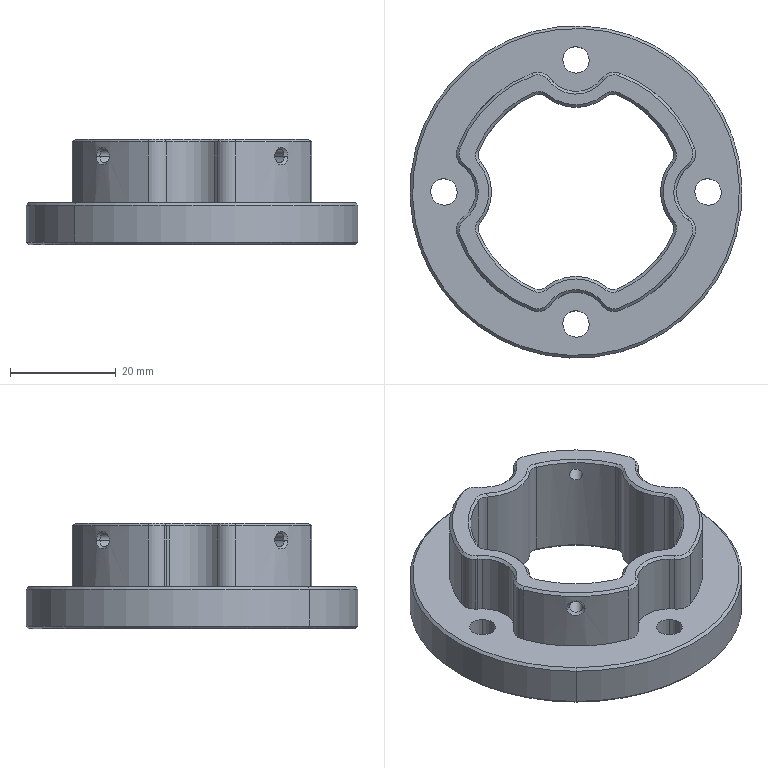NC program | NX | posted with a generic post | part box 62.9 x 62.9 x 20 mm
Lines 2530 to 3414 of 7695:
(CAVITY_MILL_COPY , TOOL : D4)
N5046 T11 M6
N5048 G54
N5050 G17 G0 G90 X-14.67 Y-5.274 S9500 M3
N5052 G43 Z30. H11
N5054 Z1.201
N5056 G94 G1 Z-0.299 F1000.
N5058 X-14.965 Y-5.264
N5060 G3 X-15.848 Y-5.732 R1.
N5062 G2 X-16.679 Y-6.883 R10.799 F2000.
N5064 G3 X-16.71 Y-7.09 R0.201
N5066 X-15.99 Y-8.591 R18.151
N5068 X-15.14 Y-9.117 R1.
N5070 G1 X-14.756 Y-9.129
N5072 Z1.201
N5074 G0 Z30.
N5076 X-14.453 Y-5.292
N5078 Z0.903
N5080 G1 Z-0.597 F1000.
N5082 X-14.749 Y-5.284
N5084 G3 X-15.629 Y-5.76 R1.
N5086 G2 X-16.524 Y-7.011 R11. F2000.
N5088 G3 X-15.747 Y-8.617 R17.95
N5090 X-14.892 Y-9.136 R1.
N5092 G1 X-14.508 Y-9.145
N5094 Z0.903
N5096 G0 Z30.
N5098 X-14.453 Y-5.292
N5100 Z0.604
N5102 G1 Z-0.896 F1000.
N5104 X-14.749 Y-5.284
N5106 G3 X-15.629 Y-5.76 R1.
N5108 G2 X-16.524 Y-7.011 R11. F2000.
N5110 G3 X-15.747 Y-8.617 R17.95
N5112 X-14.892 Y-9.136 R1.
N5114 G1 X-14.508 Y-9.145
N5116 Z0.604
N5118 G0 Z30.
N5120 X-14.453 Y-5.292
N5122 Z0.306
N5124 G1 Z-1.194 F1000.
N5126 X-14.749 Y-5.284
N5128 G3 X-15.629 Y-5.76 R1.
N5130 G2 X-16.524 Y-7.011 R11. F2000.
N5132 G3 X-15.747 Y-8.617 R17.95
N5134 X-14.892 Y-9.136 R1.
N5136 G1 X-14.508 Y-9.145
N5138 Z0.306
N5140 G0 Z30.
N5142 X-14.453 Y-5.292
N5144 Z0.007
N5146 G1 Z-1.493 F1000.
N5148 X-14.749 Y-5.284
N5150 G3 X-15.629 Y-5.76 R1.
N5152 G2 X-16.524 Y-7.011 R11. F2000.
N5154 G3 X-15.747 Y-8.617 R17.95
N5156 X-14.892 Y-9.136 R1.
N5158 G1 X-14.508 Y-9.145
N5160 Z0.007
N5162 G0 X-14.453 Y-5.292 Z-0.291
N5164 G1 Z-1.791 F1000.
N5166 X-14.749 Y-5.284
N5168 G3 X-15.629 Y-5.76 R1.
N5170 G2 X-16.524 Y-7.011 R11. F2000.
N5172 G3 X-15.747 Y-8.617 R17.95
N5174 X-14.892 Y-9.136 R1.
N5176 G1 X-14.508 Y-9.145
N5178 Z-0.291
N5180 G0 X-14.453 Y-5.292 Z-0.59
N5182 G1 Z-2.09 F1000.
N5184 X-14.749 Y-5.284
N5186 G3 X-15.629 Y-5.76 R1.
N5188 G2 X-16.524 Y-7.011 R11. F2000.
N5190 G3 X-15.747 Y-8.617 R17.95
N5192 X-14.892 Y-9.136 R1.
N5194 G1 X-14.508 Y-9.145
N5196 Z-0.59
N5198 G0 X-14.453 Y-5.292 Z-0.888
N5200 G1 Z-2.388 F1000.
N5202 X-14.749 Y-5.284
N5204 G3 X-15.629 Y-5.76 R1.
N5206 G2 X-16.524 Y-7.011 R11. F2000.
N5208 G3 X-15.747 Y-8.617 R17.95
N5210 X-14.892 Y-9.136 R1.
N5212 G1 X-14.508 Y-9.145
N5214 Z-0.888
N5216 G0 X-14.453 Y-5.292 Z-1.187
N5218 G1 Z-2.687 F1000.
N5220 X-14.749 Y-5.284
N5222 G3 X-15.629 Y-5.76 R1.
N5224 G2 X-16.524 Y-7.011 R11. F2000.
N5226 G3 X-15.747 Y-8.617 R17.95
N5228 X-14.892 Y-9.136 R1.
N5230 G1 X-14.508 Y-9.145
N5232 Z-1.187
N5234 G0 X-14.453 Y-5.292 Z-1.485
N5236 G1 Z-2.985 F1000.
N5238 X-14.749 Y-5.284
N5240 G3 X-15.629 Y-5.76 R1.
N5242 G2 X-16.524 Y-7.011 R11. F2000.
N5244 G3 X-15.747 Y-8.617 R17.95
N5246 X-14.892 Y-9.136 R1.
N5248 G1 X-14.508 Y-9.145
N5250 Z-1.485
N5252 G0 X-14.453 Y-5.292 Z-1.784
N5254 G1 Z-3.284 F1000.
N5256 X-14.749 Y-5.284
N5258 G3 X-15.629 Y-5.76 R1.
N5260 G2 X-16.524 Y-7.011 R11. F2000.
N5262 G3 X-15.747 Y-8.617 R17.95
N5264 X-14.892 Y-9.136 R1.
N5266 G1 X-14.508 Y-9.145
N5268 Z-1.784
N5270 G0 X-14.453 Y-5.292 Z-2.082
N5272 G1 Z-3.582 F1000.
N5274 X-14.749 Y-5.284
N5276 G3 X-15.629 Y-5.76 R1.
N5278 G2 X-16.524 Y-7.011 R11. F2000.
N5280 G3 X-15.747 Y-8.617 R17.95
N5282 X-14.892 Y-9.136 R1.
N5284 G1 X-14.508 Y-9.145
N5286 Z-2.082
N5288 G0 X-14.453 Y-5.292 Z-2.381
N5290 G1 Z-3.881 F1000.
N5292 X-14.749 Y-5.284
N5294 G3 X-15.629 Y-5.76 R1.
N5296 G2 X-16.524 Y-7.011 R11. F2000.
N5298 G3 X-15.747 Y-8.617 R17.95
N5300 X-14.892 Y-9.136 R1.
N5302 G1 X-14.508 Y-9.145
N5304 Z-2.381
N5306 G0 X-14.453 Y-5.292 Z-2.679
N5308 G1 Z-4.179 F1000.
N5310 X-14.749 Y-5.284
N5312 G3 X-15.629 Y-5.76 R1.
N5314 G2 X-16.524 Y-7.011 R11. F2000.
N5316 G3 X-15.747 Y-8.617 R17.95
N5318 X-14.892 Y-9.136 R1.
N5320 G1 X-14.508 Y-9.145
N5322 Z-2.679
N5324 G0 X-14.453 Y-5.292 Z-2.978
N5326 G1 Z-4.478 F1000.
N5328 X-14.749 Y-5.284
N5330 G3 X-15.629 Y-5.76 R1.
N5332 G2 X-16.524 Y-7.011 R11. F2000.
N5334 G3 X-15.747 Y-8.617 R17.95
N5336 X-14.892 Y-9.136 R1.
N5338 G1 X-14.508 Y-9.145
N5340 Z-2.978
N5342 G0 X-14.453 Y-5.292 Z-3.276
N5344 G1 Z-4.776 F1000.
N5346 X-14.749 Y-5.284
N5348 G3 X-15.629 Y-5.76 R1.
N5350 G2 X-16.524 Y-7.011 R11. F2000.
N5352 G3 X-15.747 Y-8.617 R17.95
N5354 X-14.892 Y-9.136 R1.
N5356 G1 X-14.508 Y-9.145
N5358 Z-3.276
N5360 G0 X-14.453 Y-5.292 Z-3.575
N5362 G1 Z-5.075 F1000.
N5364 X-14.749 Y-5.284
N5366 G3 X-15.629 Y-5.76 R1.
N5368 G2 X-16.524 Y-7.011 R11. F2000.
N5370 G3 X-15.747 Y-8.617 R17.95
N5372 X-14.892 Y-9.136 R1.
N5374 G1 X-14.508 Y-9.145
N5376 Z-3.575
N5378 G0 X-14.453 Y-5.292 Z-3.873
N5380 G1 Z-5.373 F1000.
N5382 X-14.749 Y-5.284
N5384 G3 X-15.629 Y-5.76 R1.
N5386 G2 X-16.524 Y-7.011 R11. F2000.
N5388 G3 X-15.747 Y-8.617 R17.95
N5390 X-14.892 Y-9.136 R1.
N5392 G1 X-14.508 Y-9.145
N5394 Z-3.873
N5396 G0 X-14.453 Y-5.292 Z-4.172
N5398 G1 Z-5.672 F1000.
N5400 X-14.749 Y-5.284
N5402 G3 X-15.629 Y-5.76 R1.
N5404 G2 X-16.524 Y-7.011 R11. F2000.
N5406 G3 X-15.747 Y-8.617 R17.95
N5408 X-14.892 Y-9.136 R1.
N5410 G1 X-14.508 Y-9.145
N5412 Z-4.172
N5414 G0 X-14.453 Y-5.292 Z-4.47
N5416 G1 Z-5.97 F1000.
N5418 X-14.749 Y-5.284
N5420 G3 X-15.629 Y-5.76 R1.
N5422 G2 X-16.524 Y-7.011 R11. F2000.
N5424 G3 X-15.747 Y-8.617 R17.95
N5426 X-14.892 Y-9.136 R1.
N5428 G1 X-14.508 Y-9.145
N5430 Z-4.47
N5432 G0 X-14.453 Y-5.292 Z-4.769
N5434 G1 Z-6.269 F1000.
N5436 X-14.749 Y-5.284
N5438 G3 X-15.629 Y-5.76 R1.
N5440 G2 X-16.524 Y-7.011 R11. F2000.
N5442 G3 X-15.747 Y-8.617 R17.95
N5444 X-14.892 Y-9.136 R1.
N5446 G1 X-14.508 Y-9.145
N5448 Z-4.769
N5450 G0 X-14.453 Y-5.292 Z-5.067
N5452 G1 Z-6.567 F1000.
N5454 X-14.749 Y-5.284
N5456 G3 X-15.629 Y-5.76 R1.
N5458 G2 X-16.524 Y-7.011 R11. F2000.
N5460 G3 X-15.747 Y-8.617 R17.95
N5462 X-14.892 Y-9.136 R1.
N5464 G1 X-14.508 Y-9.145
N5466 Z-5.067
N5468 G0 X-14.453 Y-5.292 Z-5.366
N5470 G1 Z-6.866 F1000.
N5472 X-14.749 Y-5.284
N5474 G3 X-15.629 Y-5.76 R1.
N5476 G2 X-16.524 Y-7.011 R11. F2000.
N5478 G3 X-15.747 Y-8.617 R17.95
N5480 X-14.892 Y-9.136 R1.
N5482 G1 X-14.508 Y-9.145
N5484 Z-5.366
N5486 G0 X-14.453 Y-5.292 Z-5.664
N5488 G1 Z-7.164 F1000.
N5490 X-14.749 Y-5.284
N5492 G3 X-15.629 Y-5.76 R1.
N5494 G2 X-16.524 Y-7.011 R11. F2000.
N5496 G3 X-15.747 Y-8.617 R17.95
N5498 X-14.892 Y-9.136 R1.
N5500 G1 X-14.508 Y-9.145
N5502 Z-5.664
N5504 G0 X-14.453 Y-5.292 Z-5.963
N5506 G1 Z-7.463 F1000.
N5508 X-14.749 Y-5.284
N5510 G3 X-15.629 Y-5.76 R1.
N5512 G2 X-16.524 Y-7.011 R11. F2000.
N5514 G3 X-15.747 Y-8.617 R17.95
N5516 X-14.892 Y-9.136 R1.
N5518 G1 X-14.508 Y-9.145
N5520 Z-5.963
N5522 G0 X-14.453 Y-5.292 Z-6.261
N5524 G1 Z-7.761 F1000.
N5526 X-14.749 Y-5.284
N5528 G3 X-15.629 Y-5.76 R1.
N5530 G2 X-16.524 Y-7.011 R11. F2000.
N5532 G3 X-15.747 Y-8.617 R17.95
N5534 X-14.892 Y-9.136 R1.
N5536 G1 X-14.508 Y-9.145
N5538 Z-6.261
N5540 G0 X-14.453 Y-5.292 Z-6.56
N5542 G1 Z-8.06 F1000.
N5544 X-14.749 Y-5.284
N5546 G3 X-15.629 Y-5.76 R1.
N5548 G2 X-16.524 Y-7.011 R11. F2000.
N5550 G3 X-15.747 Y-8.617 R17.95
N5552 X-14.892 Y-9.136 R1.
N5554 G1 X-14.508 Y-9.145
N5556 Z-6.56
N5558 G0 X-14.453 Y-5.292 Z-6.858
N5560 G1 Z-8.358 F1000.
N5562 X-14.749 Y-5.284
N5564 G3 X-15.629 Y-5.76 R1.
N5566 G2 X-16.524 Y-7.011 R11. F2000.
N5568 G3 X-15.747 Y-8.617 R17.95
N5570 X-14.892 Y-9.136 R1.
N5572 G1 X-14.508 Y-9.145
N5574 Z-6.858
N5576 G0 X-14.453 Y-5.292 Z-7.157
N5578 G1 Z-8.657 F1000.
N5580 X-14.749 Y-5.284
N5582 G3 X-15.629 Y-5.76 R1.
N5584 G2 X-16.524 Y-7.011 R11. F2000.
N5586 G3 X-15.747 Y-8.617 R17.95
N5588 X-14.892 Y-9.136 R1.
N5590 G1 X-14.508 Y-9.145
N5592 Z-7.157
N5594 G0 X-14.453 Y-5.292 Z-7.455
N5596 G1 Z-8.955 F1000.
N5598 X-14.749 Y-5.284
N5600 G3 X-15.629 Y-5.76 R1.
N5602 G2 X-16.524 Y-7.011 R11. F2000.
N5604 G3 X-15.747 Y-8.617 R17.95
N5606 X-14.892 Y-9.136 R1.
N5608 G1 X-14.508 Y-9.145
N5610 Z-7.455
N5612 G0 X-14.453 Y-5.292 Z-7.754
N5614 G1 Z-9.254 F1000.
N5616 X-14.749 Y-5.284
N5618 G3 X-15.629 Y-5.76 R1.
N5620 G2 X-16.524 Y-7.011 R11. F2000.
N5622 G3 X-15.747 Y-8.617 R17.95
N5624 X-14.892 Y-9.136 R1.
N5626 G1 X-14.508 Y-9.145
N5628 Z-7.754
N5630 G0 X-14.453 Y-5.292 Z-8.052
N5632 G1 Z-9.552 F1000.
N5634 X-14.749 Y-5.284
N5636 G3 X-15.629 Y-5.76 R1.
N5638 G2 X-16.524 Y-7.011 R11. F2000.
N5640 G3 X-15.747 Y-8.617 R17.95
N5642 X-14.892 Y-9.136 R1.
N5644 G1 X-14.508 Y-9.145
N5646 Z-8.052
N5648 G0 X-14.453 Y-5.292 Z-8.351
N5650 G1 Z-9.851 F1000.
N5652 X-14.749 Y-5.284
N5654 G3 X-15.629 Y-5.76 R1.
N5656 G2 X-16.524 Y-7.011 R11. F2000.
N5658 G3 X-15.747 Y-8.617 R17.95
N5660 X-14.892 Y-9.136 R1.
N5662 G1 X-14.508 Y-9.145
N5664 Z-8.351
N5666 G0 X-14.453 Y-5.292 Z-8.649
N5668 G1 Z-10.149 F1000.
N5670 X-14.749 Y-5.284
N5672 G3 X-15.629 Y-5.76 R1.
N5674 G2 X-16.524 Y-7.011 R11. F2000.
N5676 G3 X-15.747 Y-8.617 R17.95
N5678 X-14.892 Y-9.136 R1.
N5680 G1 X-14.508 Y-9.145
N5682 Z-8.649
N5684 G0 X-14.453 Y-5.292 Z-8.948
N5686 G1 Z-10.448 F1000.
N5688 X-14.749 Y-5.284
N5690 G3 X-15.629 Y-5.76 R1.
N5692 G2 X-16.524 Y-7.011 R11. F2000.
N5694 G3 X-15.747 Y-8.617 R17.95
N5696 X-14.892 Y-9.136 R1.
N5698 G1 X-14.508 Y-9.145
N5700 Z-8.948
N5702 G0 X-14.453 Y-5.292 Z-9.246
N5704 G1 Z-10.746 F1000.
N5706 X-14.749 Y-5.284
N5708 G3 X-15.629 Y-5.76 R1.
N5710 G2 X-16.524 Y-7.011 R11. F2000.
N5712 G3 X-15.747 Y-8.617 R17.95
N5714 X-14.892 Y-9.136 R1.
N5716 G1 X-14.508 Y-9.145
N5718 Z-9.246
N5720 G0 X-14.453 Y-5.292 Z-9.545
N5722 G1 Z-11.045 F1000.
N5724 X-14.749 Y-5.284
N5726 G3 X-15.629 Y-5.76 R1.
N5728 G2 X-16.524 Y-7.011 R11. F2000.
N5730 G3 X-15.747 Y-8.617 R17.95
N5732 X-14.892 Y-9.136 R1.
N5734 G1 X-14.508 Y-9.145
N5736 Z-9.545
N5738 G0 X-14.453 Y-5.292 Z-9.843
N5740 G1 Z-11.343 F1000.
N5742 X-14.749 Y-5.284
N5744 G3 X-15.629 Y-5.76 R1.
N5746 G2 X-16.524 Y-7.011 R11. F2000.
N5748 G3 X-15.747 Y-8.617 R17.95
N5750 X-14.892 Y-9.136 R1.
N5752 G1 X-14.508 Y-9.145
N5754 Z-9.843
N5756 G0 X-14.453 Y-5.292 Z-10.142
N5758 G1 Z-11.642 F1000.
N5760 X-14.749 Y-5.284
N5762 G3 X-15.629 Y-5.76 R1.
N5764 G2 X-16.524 Y-7.011 R11. F2000.
N5766 G3 X-15.747 Y-8.617 R17.95
N5768 X-14.892 Y-9.136 R1.
N5770 G1 X-14.508 Y-9.145
N5772 Z-10.142
N5774 G0 X-14.453 Y-5.292 Z-10.44
N5776 G1 Z-11.94 F1000.
N5778 X-14.749 Y-5.284
N5780 G3 X-15.629 Y-5.76 R1.
N5782 G2 X-16.524 Y-7.011 R11. F2000.
N5784 G3 X-15.747 Y-8.617 R17.95
N5786 X-14.892 Y-9.136 R1.
N5788 G1 X-14.508 Y-9.145
N5790 Z-10.44
N5792 G0 X-14.453 Y-5.292 Z-10.739
N5794 G1 Z-12.239 F1000.
N5796 X-14.749 Y-5.284
N5798 G3 X-15.629 Y-5.76 R1.
N5800 G2 X-16.524 Y-7.011 R11. F2000.
N5802 G3 X-15.747 Y-8.617 R17.95
N5804 X-14.892 Y-9.136 R1.
N5806 G1 X-14.508 Y-9.145
N5808 Z-10.739
N5810 G0 X-14.453 Y-5.292 Z-11.037
N5812 G1 Z-12.537 F1000.
N5814 X-14.749 Y-5.284
N5816 G3 X-15.629 Y-5.76 R1.
N5818 G2 X-16.524 Y-7.011 R11. F2000.
N5820 G3 X-15.747 Y-8.617 R17.95
N5822 X-14.892 Y-9.136 R1.
N5824 G1 X-14.508 Y-9.145
N5826 Z-11.037
N5828 G0 X-14.453 Y-5.292 Z-11.336
N5830 G1 Z-12.836 F1000.
N5832 X-14.749 Y-5.284
N5834 G3 X-15.629 Y-5.76 R1.
N5836 G2 X-16.524 Y-7.011 R11. F2000.
N5838 G3 X-15.747 Y-8.617 R17.95
N5840 X-14.892 Y-9.136 R1.
N5842 G1 X-14.508 Y-9.145
N5844 Z-11.336
N5846 G0 X-14.453 Y-5.292 Z-11.634
N5848 G1 Z-13.134 F1000.
N5850 X-14.749 Y-5.284
N5852 G3 X-15.629 Y-5.76 R1.
N5854 G2 X-16.524 Y-7.011 R11. F2000.
N5856 G3 X-15.747 Y-8.617 R17.95
N5858 X-14.892 Y-9.136 R1.
N5860 G1 X-14.508 Y-9.145
N5862 Z-11.634
N5864 G0 X-14.453 Y-5.292 Z-11.933
N5866 G1 Z-13.433 F1000.
N5868 X-14.749 Y-5.284
N5870 G3 X-15.629 Y-5.76 R1.
N5872 G2 X-16.524 Y-7.011 R11. F2000.
N5874 G3 X-15.747 Y-8.617 R17.95
N5876 X-14.892 Y-9.136 R1.
N5878 G1 X-14.508 Y-9.145
N5880 Z-11.933
N5882 G0 X-14.453 Y-5.292 Z-12.231
N5884 G1 Z-13.731 F1000.
N5886 X-14.749 Y-5.284
N5888 G3 X-15.629 Y-5.76 R1.
N5890 G2 X-16.524 Y-7.011 R11. F2000.
N5892 G3 X-15.747 Y-8.617 R17.95
N5894 X-14.892 Y-9.136 R1.
N5896 G1 X-14.508 Y-9.145
N5898 Z-12.231
N5900 G0 X-14.453 Y-5.292 Z-12.53
N5902 G1 Z-14.03 F1000.
N5904 X-14.749 Y-5.284
N5906 G3 X-15.629 Y-5.76 R1.
N5908 G2 X-16.524 Y-7.011 R11. F2000.
N5910 G3 X-15.747 Y-8.617 R17.95
N5912 X-14.892 Y-9.136 R1.
N5914 G1 X-14.508 Y-9.145
N5916 Z-12.53
N5918 G0 X-14.453 Y-5.292 Z-12.828
N5920 G1 Z-14.328 F1000.
N5922 X-14.749 Y-5.284
N5924 G3 X-15.629 Y-5.76 R1.
N5926 G2 X-16.524 Y-7.011 R11. F2000.
N5928 G3 X-15.747 Y-8.617 R17.95
N5930 X-14.892 Y-9.136 R1.
N5932 G1 X-14.508 Y-9.145
N5934 Z-12.828
N5936 G0 X-14.453 Y-5.292 Z-13.127
N5938 G1 Z-14.627 F1000.
N5940 X-14.749 Y-5.284
N5942 G3 X-15.629 Y-5.76 R1.
N5944 G2 X-16.524 Y-7.011 R11. F2000.
N5946 G3 X-15.747 Y-8.617 R17.95
N5948 X-14.892 Y-9.136 R1.
N5950 G1 X-14.508 Y-9.145
N5952 Z-13.127
N5954 G0 X-14.453 Y-5.292 Z-13.425
N5956 G1 Z-14.925 F1000.
N5958 X-14.749 Y-5.284
N5960 G3 X-15.629 Y-5.76 R1.
N5962 G2 X-16.524 Y-7.011 R11. F2000.
N5964 G3 X-15.747 Y-8.617 R17.95
N5966 X-14.892 Y-9.136 R1.
N5968 G1 X-14.508 Y-9.145
N5970 Z-13.425
N5972 G0 X-14.453 Y-5.292 Z-13.724
N5974 G1 Z-15.224 F1000.
N5976 X-14.749 Y-5.284
N5978 G3 X-15.629 Y-5.76 R1.
N5980 G2 X-16.524 Y-7.011 R11. F2000.
N5982 G3 X-15.747 Y-8.617 R17.95
N5984 X-14.892 Y-9.136 R1.
N5986 G1 X-14.508 Y-9.145
N5988 Z-13.724
N5990 G0 X-14.453 Y-5.292 Z-14.022
N5992 G1 Z-15.522 F1000.
N5994 X-14.749 Y-5.284
N5996 G3 X-15.629 Y-5.76 R1.
N5998 G2 X-16.524 Y-7.011 R11. F2000.
N6000 G3 X-15.747 Y-8.617 R17.95
N6002 X-14.892 Y-9.136 R1.
N6004 G1 X-14.508 Y-9.145
N6006 Z-14.022
N6008 G0 X-14.453 Y-5.292 Z-14.321
N6010 G1 Z-15.821 F1000.
N6012 X-14.749 Y-5.284
N6014 G3 X-15.629 Y-5.76 R1.
N6016 G2 X-16.524 Y-7.011 R11. F2000.
N6018 G3 X-15.747 Y-8.617 R17.95
N6020 X-14.892 Y-9.136 R1.
N6022 G1 X-14.508 Y-9.145
N6024 Z-14.321
N6026 G0 X-14.453 Y-5.292 Z-14.619
N6028 G1 Z-16.119 F1000.
N6030 X-14.749 Y-5.284
N6032 G3 X-15.629 Y-5.76 R1.
N6034 G2 X-16.524 Y-7.011 R11. F2000.
N6036 G3 X-15.747 Y-8.617 R17.95
N6038 X-14.892 Y-9.136 R1.
N6040 G1 X-14.508 Y-9.145
N6042 Z-14.619
N6044 G0 X-14.453 Y-5.292 Z-14.918
N6046 G1 Z-16.418 F1000.
N6048 X-14.749 Y-5.284
N6050 G3 X-15.629 Y-5.76 R1.
N6052 G2 X-16.524 Y-7.011 R11. F2000.
N6054 G3 X-15.747 Y-8.617 R17.95
N6056 X-14.892 Y-9.136 R1.
N6058 G1 X-14.508 Y-9.145
N6060 Z-14.918
N6062 G0 X-14.453 Y-5.292 Z-15.216
N6064 G1 Z-16.716 F1000.
N6066 X-14.749 Y-5.284
N6068 G3 X-15.629 Y-5.76 R1.
N6070 G2 X-16.524 Y-7.011 R11. F2000.
N6072 G3 X-15.747 Y-8.617 R17.95
N6074 X-14.892 Y-9.136 R1.
N6076 G1 X-14.508 Y-9.145
N6078 Z-15.216
N6080 G0 X-14.453 Y-5.292 Z-15.515
N6082 G1 Z-17.015 F1000.
N6084 X-14.749 Y-5.284
N6086 G3 X-15.629 Y-5.76 R1.
N6088 G2 X-16.524 Y-7.011 R11. F2000.
N6090 G3 X-15.747 Y-8.617 R17.95
N6092 X-14.892 Y-9.136 R1.
N6094 G1 X-14.508 Y-9.145
N6096 Z-15.515
N6098 G0 X-14.453 Y-5.292 Z-15.813
N6100 G1 Z-17.313 F1000.
N6102 X-14.749 Y-5.284
N6104 G3 X-15.629 Y-5.76 R1.
N6106 G2 X-16.524 Y-7.011 R11. F2000.
N6108 G3 X-15.747 Y-8.617 R17.95
N6110 X-14.892 Y-9.136 R1.
N6112 G1 X-14.508 Y-9.145
N6114 Z-15.813
N6116 G0 X-14.453 Y-5.292 Z-16.112
N6118 G1 Z-17.612 F1000.
N6120 X-14.749 Y-5.284
N6122 G3 X-15.629 Y-5.76 R1.
N6124 G2 X-16.524 Y-7.011 R11. F2000.
N6126 G3 X-15.747 Y-8.617 R17.95
N6128 X-14.892 Y-9.136 R1.
N6130 G1 X-14.508 Y-9.145
N6132 Z-16.112
N6134 G0 X-14.453 Y-5.292 Z-16.41
N6136 G1 Z-17.91 F1000.
N6138 X-14.749 Y-5.284
N6140 G3 X-15.629 Y-5.76 R1.
N6142 G2 X-16.524 Y-7.011 R11. F2000.
N6144 G3 X-15.747 Y-8.617 R17.95
N6146 X-14.892 Y-9.136 R1.
N6148 G1 X-14.508 Y-9.145
N6150 Z-16.41
N6152 G0 X-14.453 Y-5.292 Z-16.709
N6154 G1 Z-18.209 F1000.
N6156 X-14.749 Y-5.284
N6158 G3 X-15.629 Y-5.76 R1.
N6160 G2 X-16.524 Y-7.011 R11. F2000.
N6162 G3 X-15.747 Y-8.617 R17.95
N6164 X-14.892 Y-9.136 R1.
N6166 G1 X-14.508 Y-9.145
N6168 Z-16.709
N6170 G0 X-14.453 Y-5.292 Z-17.007
N6172 G1 Z-18.507 F1000.
N6174 X-14.749 Y-5.284
N6176 G3 X-15.629 Y-5.76 R1.
N6178 G2 X-16.524 Y-7.011 R11. F2000.
N6180 G3 X-15.747 Y-8.617 R17.95
N6182 X-14.892 Y-9.136 R1.
N6184 G1 X-14.508 Y-9.145
N6186 Z-17.007
N6188 G0 X-14.453 Y-5.292 Z-17.306
N6190 G1 Z-18.806 F1000.
N6192 X-14.749 Y-5.284
N6194 G3 X-15.629 Y-5.76 R1.
N6196 G2 X-16.524 Y-7.011 R11. F2000.
N6198 G3 X-15.747 Y-8.617 R17.95
N6200 X-14.892 Y-9.136 R1.
N6202 G1 X-14.508 Y-9.145
N6204 Z-17.306
N6206 G0 X-14.453 Y-5.292 Z-17.604
N6208 G1 Z-19.104 F1000.
N6210 X-14.749 Y-5.284
N6212 G3 X-15.629 Y-5.76 R1.
N6214 G2 X-16.524 Y-7.011 R11. F2000.
N6216 G3 X-15.747 Y-8.617 R17.95
N6218 X-14.892 Y-9.136 R1.
N6220 G1 X-14.508 Y-9.145
N6222 Z-17.604
N6224 G0 X-14.453 Y-5.292 Z-17.903
N6226 G1 Z-19.403 F1000.
N6228 X-14.749 Y-5.284
N6230 G3 X-15.629 Y-5.76 R1.
N6232 G2 X-16.524 Y-7.011 R11. F2000.
N6234 G3 X-15.747 Y-8.617 R17.95
N6236 X-14.892 Y-9.136 R1.
N6238 G1 X-14.508 Y-9.145
N6240 Z-17.903
N6242 G0 X-14.453 Y-5.292 Z-18.201
N6244 G1 Z-19.701 F1000.
N6246 X-14.749 Y-5.283
N6248 G3 X-15.628 Y-5.759 R1.
N6250 G2 X-16.524 Y-7.011 R11. F2000.
N6252 G3 X-15.744 Y-8.621 R17.95
N6254 X-14.89 Y-9.141 R1.
N6256 G1 X-14.506 Y-9.149
N6258 Z-18.201
N6260 G0 X-14.453 Y-5.292 Z-18.5
N6262 G1 Z-20. F1000.
N6264 X-14.749 Y-5.283
N6266 G3 X-15.628 Y-5.759 R1.
N6268 G2 X-16.524 Y-7.011 R11. F2000.
N6270 G3 X-15.744 Y-8.621 R17.95
N6272 X-14.89 Y-9.141 R1.
N6274 G1 X-14.506 Y-9.149
N6276 Z-18.5
N6278 G0 Z30.
N6280 X-9.129 Y-14.756
N6282 Z1.201
N6284 G1 Z-0.299 F1000.
N6286 X-9.117 Y-15.14
N6288 G3 X-8.591 Y-15.99 R1.
N6290 X-7.09 Y-16.71 R18.151 F2000.
N6292 X-6.883 Y-16.679 R0.201
N6294 G2 X-5.732 Y-15.848 R10.799
N6296 G3 X-5.264 Y-14.965 R1.
N6298 G1 X-5.274 Y-14.67
N6300 Z1.201
N6302 G0 Z30.
N6304 X-9.145 Y-14.508
N6306 Z0.903
N6308 G1 Z-0.597 F1000.
N6310 X-9.136 Y-14.892
N6312 G3 X-8.617 Y-15.747 R1.
N6314 X-7.011 Y-16.524 R17.95 F2000.
N6316 G2 X-5.76 Y-15.629 R11.
N6318 G3 X-5.284 Y-14.749 R1.
N6320 G1 X-5.292 Y-14.453
N6322 Z0.903
N6324 G0 Z30.
N6326 X-9.145 Y-14.508
N6328 Z0.604
N6330 G1 Z-0.896 F1000.
N6332 X-9.136 Y-14.892
N6334 G3 X-8.617 Y-15.747 R1.
N6336 X-7.011 Y-16.524 R17.95 F2000.
N6338 G2 X-5.76 Y-15.629 R11.
N6340 G3 X-5.284 Y-14.749 R1.
N6342 G1 X-5.292 Y-14.453
N6344 Z0.604
N6346 G0 Z30.
N6348 X-9.145 Y-14.508
N6350 Z0.306
N6352 G1 Z-1.194 F1000.
N6354 X-9.136 Y-14.892
N6356 G3 X-8.617 Y-15.747 R1.
N6358 X-7.011 Y-16.524 R17.95 F2000.
N6360 G2 X-5.76 Y-15.629 R11.
N6362 G3 X-5.284 Y-14.749 R1.
N6364 G1 X-5.292 Y-14.453
N6366 Z0.306
N6368 G0 Z30.
N6370 X-9.145 Y-14.508
N6372 Z0.007
N6374 G1 Z-1.493 F1000.
N6376 X-9.136 Y-14.892
N6378 G3 X-8.617 Y-15.747 R1.
N6380 X-7.011 Y-16.524 R17.95 F2000.
N6382 G2 X-5.76 Y-15.629 R11.
N6384 G3 X-5.284 Y-14.749 R1.
N6386 G1 X-5.292 Y-14.453
N6388 Z0.007
N6390 G0 X-9.145 Y-14.508 Z-0.291
N6392 G1 Z-1.791 F1000.
N6394 X-9.136 Y-14.892
N6396 G3 X-8.617 Y-15.747 R1.
N6398 X-7.011 Y-16.524 R17.95 F2000.
N6400 G2 X-5.76 Y-15.629 R11.
N6402 G3 X-5.284 Y-14.749 R1.
N6404 G1 X-5.292 Y-14.453
N6406 Z-0.291
N6408 G0 X-9.145 Y-14.508 Z-0.59
N6410 G1 Z-2.09 F1000.
N6412 X-9.136 Y-14.892
N6414 G3 X-8.617 Y-15.747 R1.
N6416 X-7.011 Y-16.524 R17.95 F2000.
N6418 G2 X-5.76 Y-15.629 R11.
N6420 G3 X-5.284 Y-14.749 R1.
N6422 G1 X-5.292 Y-14.453
N6424 Z-0.59
N6426 G0 X-9.145 Y-14.508 Z-0.888
N6428 G1 Z-2.388 F1000.
N6430 X-9.136 Y-14.892
N6432 G3 X-8.617 Y-15.747 R1.
N6434 X-7.011 Y-16.524 R17.95 F2000.
N6436 G2 X-5.76 Y-15.629 R11.
N6438 G3 X-5.284 Y-14.749 R1.
N6440 G1 X-5.292 Y-14.453
N6442 Z-0.888
N6444 G0 X-9.145 Y-14.508 Z-1.187
N6446 G1 Z-2.687 F1000.
N6448 X-9.136 Y-14.892
N6450 G3 X-8.617 Y-15.747 R1.
N6452 X-7.011 Y-16.524 R17.95 F2000.
N6454 G2 X-5.76 Y-15.629 R11.
N6456 G3 X-5.284 Y-14.749 R1.
N6458 G1 X-5.292 Y-14.453
N6460 Z-1.187
N6462 G0 X-9.145 Y-14.508 Z-1.485
N6464 G1 Z-2.985 F1000.
N6466 X-9.136 Y-14.892
N6468 G3 X-8.617 Y-15.747 R1.
N6470 X-7.011 Y-16.524 R17.95 F2000.
N6472 G2 X-5.76 Y-15.629 R11.
N6474 G3 X-5.284 Y-14.749 R1.
N6476 G1 X-5.292 Y-14.453
N6478 Z-1.485
N6480 G0 X-9.145 Y-14.508 Z-1.784
N6482 G1 Z-3.284 F1000.
N6484 X-9.136 Y-14.892
N6486 G3 X-8.617 Y-15.747 R1.
N6488 X-7.011 Y-16.524 R17.95 F2000.
N6490 G2 X-5.76 Y-15.629 R11.
N6492 G3 X-5.284 Y-14.749 R1.
N6494 G1 X-5.292 Y-14.453
N6496 Z-1.784
N6498 G0 X-9.145 Y-14.508 Z-2.082
N6500 G1 Z-3.582 F1000.
N6502 X-9.136 Y-14.892
N6504 G3 X-8.617 Y-15.747 R1.
N6506 X-7.011 Y-16.524 R17.95 F2000.
N6508 G2 X-5.76 Y-15.629 R11.
N6510 G3 X-5.284 Y-14.749 R1.
N6512 G1 X-5.292 Y-14.453
N6514 Z-2.082
N6516 G0 X-9.145 Y-14.508 Z-2.381
N6518 G1 Z-3.881 F1000.
N6520 X-9.136 Y-14.892
N6522 G3 X-8.617 Y-15.747 R1.
N6524 X-7.011 Y-16.524 R17.95 F2000.
N6526 G2 X-5.76 Y-15.629 R11.
N6528 G3 X-5.284 Y-14.749 R1.
N6530 G1 X-5.292 Y-14.453
N6532 Z-2.381
N6534 G0 X-9.145 Y-14.508 Z-2.679
N6536 G1 Z-4.179 F1000.
N6538 X-9.136 Y-14.892
N6540 G3 X-8.617 Y-15.747 R1.
N6542 X-7.011 Y-16.524 R17.95 F2000.
N6544 G2 X-5.76 Y-15.629 R11.
N6546 G3 X-5.284 Y-14.749 R1.
N6548 G1 X-5.292 Y-14.453
N6550 Z-2.679
N6552 G0 X-9.145 Y-14.508 Z-2.978
N6554 G1 Z-4.478 F1000.
N6556 X-9.136 Y-14.892
N6558 G3 X-8.617 Y-15.747 R1.
N6560 X-7.011 Y-16.524 R17.95 F2000.
N6562 G2 X-5.76 Y-15.629 R11.
N6564 G3 X-5.284 Y-14.749 R1.
N6566 G1 X-5.292 Y-14.453
N6568 Z-2.978
N6570 G0 X-9.145 Y-14.508 Z-3.276
N6572 G1 Z-4.776 F1000.
N6574 X-9.136 Y-14.892
N6576 G3 X-8.617 Y-15.747 R1.
N6578 X-7.011 Y-16.524 R17.95 F2000.
N6580 G2 X-5.76 Y-15.629 R11.
N6582 G3 X-5.284 Y-14.749 R1.
N6584 G1 X-5.292 Y-14.453
N6586 Z-3.276
N6588 G0 X-9.145 Y-14.508 Z-3.575
N6590 G1 Z-5.075 F1000.
N6592 X-9.136 Y-14.892
N6594 G3 X-8.617 Y-15.747 R1.
N6596 X-7.011 Y-16.524 R17.95 F2000.
N6598 G2 X-5.76 Y-15.629 R11.
N6600 G3 X-5.284 Y-14.749 R1.
N6602 G1 X-5.292 Y-14.453
N6604 Z-3.575
N6606 G0 X-9.145 Y-14.508 Z-3.873
N6608 G1 Z-5.373 F1000.
N6610 X-9.136 Y-14.892
N6612 G3 X-8.617 Y-15.747 R1.
N6614 X-7.011 Y-16.524 R17.95 F2000.
N6616 G2 X-5.76 Y-15.629 R11.
N6618 G3 X-5.284 Y-14.749 R1.
N6620 G1 X-5.292 Y-14.453
N6622 Z-3.873
N6624 G0 X-9.145 Y-14.508 Z-4.172
N6626 G1 Z-5.672 F1000.
N6628 X-9.136 Y-14.892
N6630 G3 X-8.617 Y-15.747 R1.
N6632 X-7.011 Y-16.524 R17.95 F2000.
N6634 G2 X-5.76 Y-15.629 R11.
N6636 G3 X-5.284 Y-14.749 R1.
N6638 G1 X-5.292 Y-14.453
N6640 Z-4.172
N6642 G0 X-9.145 Y-14.508 Z-4.47
N6644 G1 Z-5.97 F1000.
N6646 X-9.136 Y-14.892
N6648 G3 X-8.617 Y-15.747 R1.
N6650 X-7.011 Y-16.524 R17.95 F2000.
N6652 G2 X-5.76 Y-15.629 R11.
N6654 G3 X-5.284 Y-14.749 R1.
N6656 G1 X-5.292 Y-14.453
N6658 Z-4.47
N6660 G0 X-9.145 Y-14.508 Z-4.769
N6662 G1 Z-6.269 F1000.
N6664 X-9.136 Y-14.892
N6666 G3 X-8.617 Y-15.747 R1.
N6668 X-7.011 Y-16.524 R17.95 F2000.
N6670 G2 X-5.76 Y-15.629 R11.
N6672 G3 X-5.284 Y-14.749 R1.
N6674 G1 X-5.292 Y-14.453
N6676 Z-4.769
N6678 G0 X-9.145 Y-14.508 Z-5.067
N6680 G1 Z-6.567 F1000.
N6682 X-9.136 Y-14.892
N6684 G3 X-8.617 Y-15.747 R1.
N6686 X-7.011 Y-16.524 R17.95 F2000.
N6688 G2 X-5.76 Y-15.629 R11.
N6690 G3 X-5.284 Y-14.749 R1.
N6692 G1 X-5.292 Y-14.453
N6694 Z-5.067
N6696 G0 X-9.145 Y-14.508 Z-5.366
N6698 G1 Z-6.866 F1000.
N6700 X-9.136 Y-14.892
N6702 G3 X-8.617 Y-15.747 R1.
N6704 X-7.011 Y-16.524 R17.95 F2000.
N6706 G2 X-5.76 Y-15.629 R11.
N6708 G3 X-5.284 Y-14.749 R1.
N6710 G1 X-5.292 Y-14.453
N6712 Z-5.366
N6714 G0 X-9.145 Y-14.508 Z-5.664
N6716 G1 Z-7.164 F1000.
N6718 X-9.136 Y-14.892
N6720 G3 X-8.617 Y-15.747 R1.
N6722 X-7.011 Y-16.524 R17.95 F2000.
N6724 G2 X-5.76 Y-15.629 R11.
N6726 G3 X-5.284 Y-14.749 R1.
N6728 G1 X-5.292 Y-14.453
N6730 Z-5.664
N6732 G0 X-9.145 Y-14.508 Z-5.963
N6734 G1 Z-7.463 F1000.
N6736 X-9.136 Y-14.892
N6738 G3 X-8.617 Y-15.747 R1.
N6740 X-7.011 Y-16.524 R17.95 F2000.
N6742 G2 X-5.76 Y-15.629 R11.
N6744 G3 X-5.284 Y-14.749 R1.
N6746 G1 X-5.292 Y-14.453
N6748 Z-5.963
N6750 G0 X-9.145 Y-14.508 Z-6.261
N6752 G1 Z-7.761 F1000.
N6754 X-9.136 Y-14.892
N6756 G3 X-8.617 Y-15.747 R1.
N6758 X-7.011 Y-16.524 R17.95 F2000.
N6760 G2 X-5.76 Y-15.629 R11.
N6762 G3 X-5.284 Y-14.749 R1.
N6764 G1 X-5.292 Y-14.453
N6766 Z-6.261
N6768 G0 X-9.145 Y-14.508 Z-6.56
N6770 G1 Z-8.06 F1000.
N6772 X-9.136 Y-14.892
N6774 G3 X-8.617 Y-15.747 R1.
N6776 X-7.011 Y-16.524 R17.95 F2000.
N6778 G2 X-5.76 Y-15.629 R11.
N6780 G3 X-5.284 Y-14.749 R1.
N6782 G1 X-5.292 Y-14.453
N6784 Z-6.56
N6786 G0 X-9.145 Y-14.508 Z-6.858
N6788 G1 Z-8.358 F1000.
N6790 X-9.136 Y-14.892
N6792 G3 X-8.617 Y-15.747 R1.
N6794 X-7.011 Y-16.524 R17.95 F2000.
N6796 G2 X-5.76 Y-15.629 R11.
N6798 G3 X-5.284 Y-14.749 R1.
N6800 G1 X-5.292 Y-14.453
N6802 Z-6.858
N6804 G0 X-9.145 Y-14.508 Z-7.157
N6806 G1 Z-8.657 F1000.
N6808 X-9.136 Y-14.892